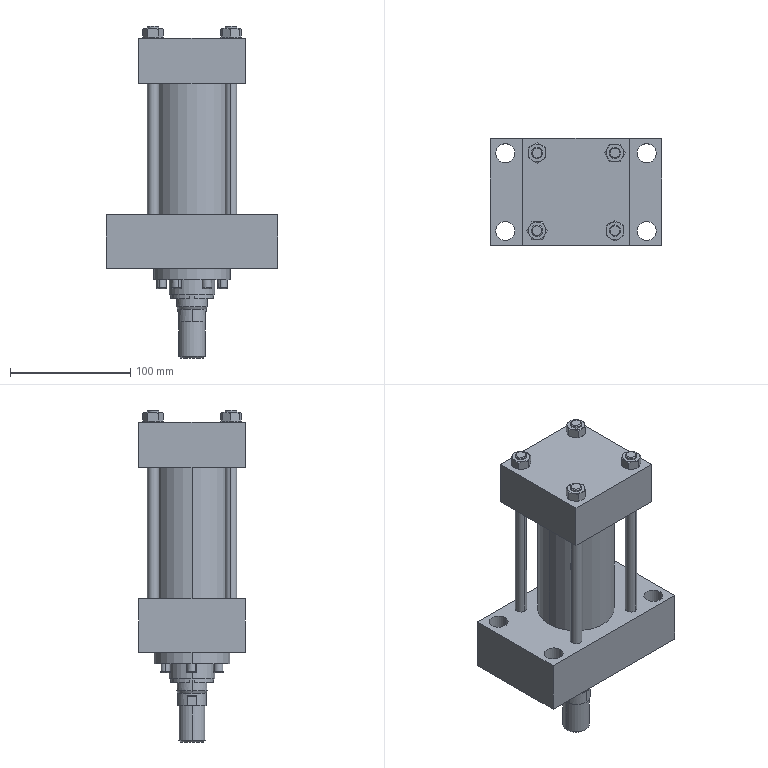Part | STEP file | 4-20.sldasm-Part-125 | 1 solid | 179 faces | box 142.875 x 88.9 x 276.19 mm | volume 1282545 mm3 | plane 75 | cylinder 64 | cone 28 | torus 12 | commonest cylinder face diameters 9.52 x16 7.937 x12 8.1 x8 15.875 x8 25.81 x4 36.07 x4